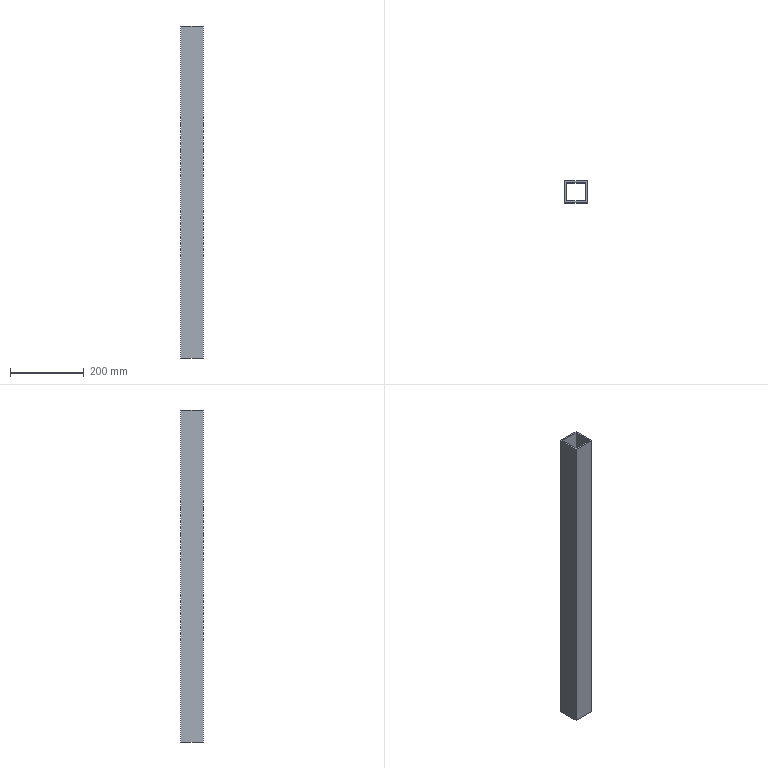Part | STEP file | Mirror slider 13 | 1 solid | 10 faces | box 60 x 60 x 900 mm | volume 990000 mm3 | plane 10
STEP:
#1=CARTESIAN_POINT('',(-30.,30.,0.));
#2=VERTEX_POINT('',#1);
#3=CARTESIAN_POINT('',(30.,30.,0.));
#4=VERTEX_POINT('',#3);
#5=CARTESIAN_POINT('',(-30.,30.,0.));
#6=DIRECTION('',(1.,0.,0.));
#7=VECTOR('',#6,1000.);
#8=LINE('',#5,#7);
#9=EDGE_CURVE('',#2,#4,#8,.T.);
#10=ORIENTED_EDGE('',*,*,#9,.T.);
#11=CARTESIAN_POINT('',(30.,30.,-900.));
#12=VERTEX_POINT('',#11);
#13=CARTESIAN_POINT('',(30.,30.,-900.));
#14=DIRECTION('',(0.,0.,1.));
#15=VECTOR('',#14,1000.);
#16=LINE('',#13,#15);
#17=EDGE_CURVE('',#12,#4,#16,.T.);
#18=ORIENTED_EDGE('',*,*,#17,.F.);
#19=CARTESIAN_POINT('',(-30.,30.,-900.));
#20=VERTEX_POINT('',#19);
#21=CARTESIAN_POINT('',(-30.,30.,-900.));
#22=DIRECTION('',(1.,0.,0.));
#23=VECTOR('',#22,1000.);
#24=LINE('',#21,#23);
#25=EDGE_CURVE('',#20,#12,#24,.T.);
#26=ORIENTED_EDGE('',*,*,#25,.F.);
#27=CARTESIAN_POINT('',(-30.,30.,-900.));
#28=DIRECTION('',(0.,0.,1.));
#29=VECTOR('',#28,1000.);
#30=LINE('',#27,#29);
#31=EDGE_CURVE('',#20,#2,#30,.T.);
#32=ORIENTED_EDGE('',*,*,#31,.T.);
#33=EDGE_LOOP('',(#10,#18,#26,#32));
#34=FACE_OUTER_BOUND('',#33,.T.);
#35=CARTESIAN_POINT('',(-30.,30.,-900.));
#36=DIRECTION('',(0.,1.,0.));
#37=DIRECTION('',(0.,0.,-1.));
#38=AXIS2_PLACEMENT_3D('',#35,#36,#37);
#39=PLANE('',#38);
#40=ADVANCED_FACE('',(#34),#39,.T.);
#41=CARTESIAN_POINT('',(-30.,-30.,0.));
#42=VERTEX_POINT('',#41);
#43=CARTESIAN_POINT('',(-30.,30.,0.));
#44=DIRECTION('',(0.,-1.,0.));
#45=VECTOR('',#44,1000.);
#46=LINE('',#43,#45);
#47=EDGE_CURVE('',#2,#42,#46,.T.);
#48=ORIENTED_EDGE('',*,*,#47,.F.);
#49=ORIENTED_EDGE('',*,*,#31,.F.);
#50=CARTESIAN_POINT('',(-30.,-30.,-900.));
#51=VERTEX_POINT('',#50);
#52=CARTESIAN_POINT('',(-30.,30.,-900.));
#53=DIRECTION('',(0.,-1.,0.));
#54=VECTOR('',#53,1000.);
#55=LINE('',#52,#54);
#56=EDGE_CURVE('',#20,#51,#55,.T.);
#57=ORIENTED_EDGE('',*,*,#56,.T.);
#58=CARTESIAN_POINT('',(-30.,-30.,-900.));
#59=DIRECTION('',(0.,0.,1.));
#60=VECTOR('',#59,1000.);
#61=LINE('',#58,#60);
#62=EDGE_CURVE('',#51,#42,#61,.T.);
#63=ORIENTED_EDGE('',*,*,#62,.T.);
#64=EDGE_LOOP('',(#48,#49,#57,#63));
#65=FACE_OUTER_BOUND('',#64,.T.);
#66=CARTESIAN_POINT('',(-30.,30.,-900.));
#67=DIRECTION('',(1.,0.,0.));
#68=DIRECTION('',(0.,1.,0.));
#69=AXIS2_PLACEMENT_3D('',#66,#67,#68);
#70=PLANE('',#69);
#71=ADVANCED_FACE('',(#65),#70,.F.);
#72=CARTESIAN_POINT('',(30.,-30.,0.));
#73=VERTEX_POINT('',#72);
#74=CARTESIAN_POINT('',(-30.,-30.,0.));
#75=DIRECTION('',(1.,0.,0.));
#76=VECTOR('',#75,1000.);
#77=LINE('',#74,#76);
#78=EDGE_CURVE('',#42,#73,#77,.T.);
#79=ORIENTED_EDGE('',*,*,#78,.F.);
#80=ORIENTED_EDGE('',*,*,#62,.F.);
#81=CARTESIAN_POINT('',(30.,-30.,-900.));
#82=VERTEX_POINT('',#81);
#83=CARTESIAN_POINT('',(-30.,-30.,-900.));
#84=DIRECTION('',(1.,0.,0.));
#85=VECTOR('',#84,1000.);
#86=LINE('',#83,#85);
#87=EDGE_CURVE('',#51,#82,#86,.T.);
#88=ORIENTED_EDGE('',*,*,#87,.T.);
#89=CARTESIAN_POINT('',(30.,-30.,-900.));
#90=DIRECTION('',(0.,0.,1.));
#91=VECTOR('',#90,1000.);
#92=LINE('',#89,#91);
#93=EDGE_CURVE('',#82,#73,#92,.T.);
#94=ORIENTED_EDGE('',*,*,#93,.T.);
#95=EDGE_LOOP('',(#79,#80,#88,#94));
#96=FACE_OUTER_BOUND('',#95,.T.);
#97=CARTESIAN_POINT('',(-30.,-30.,-900.));
#98=DIRECTION('',(0.,1.,0.));
#99=DIRECTION('',(0.,0.,-1.));
#100=AXIS2_PLACEMENT_3D('',#97,#98,#99);
#101=PLANE('',#100);
#102=ADVANCED_FACE('',(#96),#101,.F.);
#103=CARTESIAN_POINT('',(30.,30.,0.));
#104=DIRECTION('',(0.,-1.,0.));
#105=VECTOR('',#104,1000.);
#106=LINE('',#103,#105);
#107=EDGE_CURVE('',#4,#73,#106,.T.);
#108=ORIENTED_EDGE('',*,*,#107,.T.);
#109=ORIENTED_EDGE('',*,*,#93,.F.);
#110=CARTESIAN_POINT('',(30.,30.,-900.));
#111=DIRECTION('',(0.,-1.,0.));
#112=VECTOR('',#111,1000.);
#113=LINE('',#110,#112);
#114=EDGE_CURVE('',#12,#82,#113,.T.);
#115=ORIENTED_EDGE('',*,*,#114,.F.);
#116=ORIENTED_EDGE('',*,*,#17,.T.);
#117=EDGE_LOOP('',(#108,#109,#115,#116));
#118=FACE_OUTER_BOUND('',#117,.T.);
#119=CARTESIAN_POINT('',(30.,30.,-900.));
#120=DIRECTION('',(1.,0.,0.));
#121=DIRECTION('',(0.,1.,0.));
#122=AXIS2_PLACEMENT_3D('',#119,#120,#121);
#123=PLANE('',#122);
#124=ADVANCED_FACE('',(#118),#123,.T.);
#125=CARTESIAN_POINT('',(-25.,25.,-900.));
#126=VERTEX_POINT('',#125);
#127=CARTESIAN_POINT('',(-25.,-25.,-900.));
#128=VERTEX_POINT('',#127);
#129=CARTESIAN_POINT('',(-25.,0.,-900.));
#130=DIRECTION('',(0.,-1.,0.));
#131=VECTOR('',#130,1000.);
#132=LINE('',#129,#131);
#133=EDGE_CURVE('',#126,#128,#132,.T.);
#134=ORIENTED_EDGE('',*,*,#133,.T.);
#135=CARTESIAN_POINT('',(25.,-25.,-900.));
#136=VERTEX_POINT('',#135);
#137=CARTESIAN_POINT('',(0.,-25.,-900.));
#138=DIRECTION('',(1.,0.,0.));
#139=VECTOR('',#138,1000.);
#140=LINE('',#137,#139);
#141=EDGE_CURVE('',#128,#136,#140,.T.);
#142=ORIENTED_EDGE('',*,*,#141,.T.);
#143=CARTESIAN_POINT('',(25.,25.,-900.));
#144=VERTEX_POINT('',#143);
#145=CARTESIAN_POINT('',(25.,0.,-900.));
#146=DIRECTION('',(0.,-1.,0.));
#147=VECTOR('',#146,1000.);
#148=LINE('',#145,#147);
#149=EDGE_CURVE('',#144,#136,#148,.T.);
#150=ORIENTED_EDGE('',*,*,#149,.F.);
#151=CARTESIAN_POINT('',(0.,25.,-900.));
#152=DIRECTION('',(1.,0.,0.));
#153=VECTOR('',#152,1000.);
#154=LINE('',#151,#153);
#155=EDGE_CURVE('',#126,#144,#154,.T.);
#156=ORIENTED_EDGE('',*,*,#155,.F.);
#157=EDGE_LOOP('',(#134,#142,#150,#156));
#158=FACE_BOUND('',#157,.T.);
#159=ORIENTED_EDGE('',*,*,#25,.T.);
#160=ORIENTED_EDGE('',*,*,#114,.T.);
#161=ORIENTED_EDGE('',*,*,#87,.F.);
#162=ORIENTED_EDGE('',*,*,#56,.F.);
#163=EDGE_LOOP('',(#159,#160,#161,#162));
#164=FACE_OUTER_BOUND('',#163,.T.);
#165=CARTESIAN_POINT('',(0.,0.,-900.));
#166=DIRECTION('',(0.,0.,1.));
#167=DIRECTION('',(-1.,0.,0.));
#168=AXIS2_PLACEMENT_3D('',#165,#166,#167);
#169=PLANE('',#168);
#170=ADVANCED_FACE('',(#158,#164),#169,.F.);
#171=CARTESIAN_POINT('',(-25.,25.,0.));
#172=VERTEX_POINT('',#171);
#173=CARTESIAN_POINT('',(25.,25.,0.));
#174=VERTEX_POINT('',#173);
#175=CARTESIAN_POINT('',(0.,25.,0.));
#176=DIRECTION('',(1.,0.,0.));
#177=VECTOR('',#176,1000.);
#178=LINE('',#175,#177);
#179=EDGE_CURVE('',#172,#174,#178,.T.);
#180=ORIENTED_EDGE('',*,*,#179,.T.);
#181=CARTESIAN_POINT('',(25.,-25.,0.));
#182=VERTEX_POINT('',#181);
#183=CARTESIAN_POINT('',(25.,0.,0.));
#184=DIRECTION('',(0.,-1.,0.));
#185=VECTOR('',#184,1000.);
#186=LINE('',#183,#185);
#187=EDGE_CURVE('',#174,#182,#186,.T.);
#188=ORIENTED_EDGE('',*,*,#187,.T.);
#189=CARTESIAN_POINT('',(-25.,-25.,0.));
#190=VERTEX_POINT('',#189);
#191=CARTESIAN_POINT('',(0.,-25.,0.));
#192=DIRECTION('',(1.,0.,0.));
#193=VECTOR('',#192,1000.);
#194=LINE('',#191,#193);
#195=EDGE_CURVE('',#190,#182,#194,.T.);
#196=ORIENTED_EDGE('',*,*,#195,.F.);
#197=CARTESIAN_POINT('',(-25.,0.,0.));
#198=DIRECTION('',(0.,-1.,0.));
#199=VECTOR('',#198,1000.);
#200=LINE('',#197,#199);
#201=EDGE_CURVE('',#172,#190,#200,.T.);
#202=ORIENTED_EDGE('',*,*,#201,.F.);
#203=EDGE_LOOP('',(#180,#188,#196,#202));
#204=FACE_BOUND('',#203,.T.);
#205=ORIENTED_EDGE('',*,*,#9,.F.);
#206=ORIENTED_EDGE('',*,*,#47,.T.);
#207=ORIENTED_EDGE('',*,*,#78,.T.);
#208=ORIENTED_EDGE('',*,*,#107,.F.);
#209=EDGE_LOOP('',(#205,#206,#207,#208));
#210=FACE_OUTER_BOUND('',#209,.T.);
#211=CARTESIAN_POINT('',(0.,0.,0.));
#212=DIRECTION('',(0.,0.,1.));
#213=DIRECTION('',(-1.,0.,0.));
#214=AXIS2_PLACEMENT_3D('',#211,#212,#213);
#215=PLANE('',#214);
#216=ADVANCED_FACE('',(#204,#210),#215,.T.);
#217=ORIENTED_EDGE('',*,*,#179,.F.);
#218=CARTESIAN_POINT('',(-25.,25.,-900.));
#219=DIRECTION('',(0.,0.,1.));
#220=VECTOR('',#219,1000.);
#221=LINE('',#218,#220);
#222=EDGE_CURVE('',#126,#172,#221,.T.);
#223=ORIENTED_EDGE('',*,*,#222,.F.);
#224=ORIENTED_EDGE('',*,*,#155,.T.);
#225=CARTESIAN_POINT('',(25.,25.,-900.));
#226=DIRECTION('',(0.,0.,1.));
#227=VECTOR('',#226,1000.);
#228=LINE('',#225,#227);
#229=EDGE_CURVE('',#144,#174,#228,.T.);
#230=ORIENTED_EDGE('',*,*,#229,.T.);
#231=EDGE_LOOP('',(#217,#223,#224,#230));
#232=FACE_OUTER_BOUND('',#231,.T.);
#233=CARTESIAN_POINT('',(0.,25.,-900.));
#234=DIRECTION('',(0.,1.,0.));
#235=DIRECTION('',(0.,0.,-1.));
#236=AXIS2_PLACEMENT_3D('',#233,#234,#235);
#237=PLANE('',#236);
#238=ADVANCED_FACE('',(#232),#237,.F.);
#239=ORIENTED_EDGE('',*,*,#201,.T.);
#240=CARTESIAN_POINT('',(-25.,-25.,-900.));
#241=DIRECTION('',(0.,0.,1.));
#242=VECTOR('',#241,1000.);
#243=LINE('',#240,#242);
#244=EDGE_CURVE('',#128,#190,#243,.T.);
#245=ORIENTED_EDGE('',*,*,#244,.F.);
#246=ORIENTED_EDGE('',*,*,#133,.F.);
#247=ORIENTED_EDGE('',*,*,#222,.T.);
#248=EDGE_LOOP('',(#239,#245,#246,#247));
#249=FACE_OUTER_BOUND('',#248,.T.);
#250=CARTESIAN_POINT('',(-25.,0.,-900.));
#251=DIRECTION('',(1.,0.,0.));
#252=DIRECTION('',(0.,1.,0.));
#253=AXIS2_PLACEMENT_3D('',#250,#251,#252);
#254=PLANE('',#253);
#255=ADVANCED_FACE('',(#249),#254,.T.);
#256=ORIENTED_EDGE('',*,*,#195,.T.);
#257=CARTESIAN_POINT('',(25.,-25.,-900.));
#258=DIRECTION('',(0.,0.,1.));
#259=VECTOR('',#258,1000.);
#260=LINE('',#257,#259);
#261=EDGE_CURVE('',#136,#182,#260,.T.);
#262=ORIENTED_EDGE('',*,*,#261,.F.);
#263=ORIENTED_EDGE('',*,*,#141,.F.);
#264=ORIENTED_EDGE('',*,*,#244,.T.);
#265=EDGE_LOOP('',(#256,#262,#263,#264));
#266=FACE_OUTER_BOUND('',#265,.T.);
#267=CARTESIAN_POINT('',(0.,-25.,-900.));
#268=DIRECTION('',(0.,1.,0.));
#269=DIRECTION('',(0.,0.,-1.));
#270=AXIS2_PLACEMENT_3D('',#267,#268,#269);
#271=PLANE('',#270);
#272=ADVANCED_FACE('',(#266),#271,.T.);
#273=ORIENTED_EDGE('',*,*,#187,.F.);
#274=ORIENTED_EDGE('',*,*,#229,.F.);
#275=ORIENTED_EDGE('',*,*,#149,.T.);
#276=ORIENTED_EDGE('',*,*,#261,.T.);
#277=EDGE_LOOP('',(#273,#274,#275,#276));
#278=FACE_OUTER_BOUND('',#277,.T.);
#279=CARTESIAN_POINT('',(25.,0.,-900.));
#280=DIRECTION('',(1.,0.,0.));
#281=DIRECTION('',(0.,1.,0.));
#282=AXIS2_PLACEMENT_3D('',#279,#280,#281);
#283=PLANE('',#282);
#284=ADVANCED_FACE('',(#278),#283,.F.);
#285=CLOSED_SHELL('',(#40,#71,#102,#124,#170,#216,#238,#255,#272,#284));
#286=MANIFOLD_SOLID_BREP('',#285);
#287=CARTESIAN_POINT('',(0.,0.,0.));
#288=DIRECTION('',(0.,0.,1.));
#289=DIRECTION('',(1.,0.,0.));
#290=AXIS2_PLACEMENT_3D('',#287,#288,#289);
#291=(LENGTH_UNIT()NAMED_UNIT(*)SI_UNIT(.MILLI.,.METRE.));
#292=UNCERTAINTY_MEASURE_WITH_UNIT(LENGTH_MEASURE(0.00001),#291,'','');
#293=(NAMED_UNIT(*)PLANE_ANGLE_UNIT()SI_UNIT($,.RADIAN.));
#294=(NAMED_UNIT(*)SI_UNIT($,.STERADIAN.)SOLID_ANGLE_UNIT());
#295=(GEOMETRIC_REPRESENTATION_CONTEXT(3)GLOBAL_UNCERTAINTY_ASSIGNED_CONTEXT((#292))GLOBAL_UNIT_ASSIGNED_CONTEXT((#291,#293,#294))REPRESENTATION_CONTEXT('',''));
#296=ADVANCED_BREP_SHAPE_REPRESENTATION('',(#286,#290),#295);